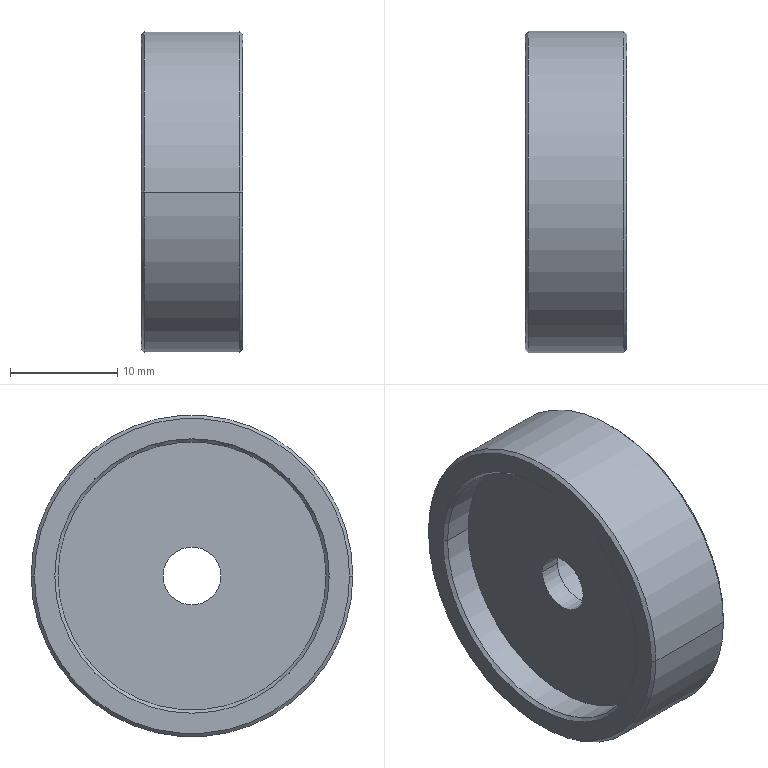Part | NX | 1 solid | 20 faces | box 9.5 x 30 x 30 mm | volume 4864 mm3 | cylinder 8 | cone 8 | plane 4 | commonest cylinder face diameters 5.4 x2 9.5 x2 25 x2 30 x2
STEP:
#1=CARTESIAN_POINT('',(215.3,157.591,-308.31));
#2=VERTEX_POINT('',#1);
#3=CARTESIAN_POINT('',(215.3,127.591,-308.31));
#4=VERTEX_POINT('',#3);
#5=CARTESIAN_POINT('',(215.3,142.591,-308.31));
#6=DIRECTION('',(-1.,0.,0.));
#7=DIRECTION('',(0.,-1.,0.));
#8=AXIS2_PLACEMENT_3D('',#5,#6,#7);
#9=CIRCLE('',#8,15.);
#10=EDGE_CURVE('',#2,#4,#9,.T.);
#11=ORIENTED_EDGE('',*,*,#10,.T.);
#12=CARTESIAN_POINT('',(206.4,127.591,-308.31));
#13=VERTEX_POINT('',#12);
#14=CARTESIAN_POINT('',(208.1,127.591,-308.31));
#15=DIRECTION('',(1.,0.,0.));
#16=VECTOR('',#15,1000.);
#17=LINE('',#14,#16);
#18=EDGE_CURVE('',#4,#13,#17,.F.);
#19=ORIENTED_EDGE('',*,*,#18,.T.);
#20=CARTESIAN_POINT('',(206.4,157.591,-308.31));
#21=VERTEX_POINT('',#20);
#22=CARTESIAN_POINT('',(206.4,142.591,-308.31));
#23=DIRECTION('',(1.,0.,0.));
#24=DIRECTION('',(0.,1.,0.));
#25=AXIS2_PLACEMENT_3D('',#22,#23,#24);
#26=CIRCLE('',#25,15.);
#27=EDGE_CURVE('',#13,#21,#26,.T.);
#28=ORIENTED_EDGE('',*,*,#27,.T.);
#29=CARTESIAN_POINT('',(208.1,157.591,-308.31));
#30=DIRECTION('',(1.,0.,0.));
#31=VECTOR('',#30,1000.);
#32=LINE('',#29,#31);
#33=EDGE_CURVE('',#2,#21,#32,.F.);
#34=ORIENTED_EDGE('',*,*,#33,.F.);
#35=EDGE_LOOP('',(#11,#19,#28,#34));
#36=FACE_BOUND('',#35,.T.);
#37=CARTESIAN_POINT('',(208.1,142.591,-308.31));
#38=DIRECTION('',(1.,0.,0.));
#39=DIRECTION('',(0.,1.,0.));
#40=AXIS2_PLACEMENT_3D('',#37,#38,#39);
#41=CYLINDRICAL_SURFACE('',#40,15.);
#42=ADVANCED_FACE('',(#36),#41,.T.);
#43=CARTESIAN_POINT('',(206.1,127.891,-308.31));
#44=VERTEX_POINT('',#43);
#45=CARTESIAN_POINT('',(206.1,157.291,-308.31));
#46=VERTEX_POINT('',#45);
#47=CARTESIAN_POINT('',(206.1,142.591,-308.31));
#48=DIRECTION('',(1.,0.,0.));
#49=DIRECTION('',(0.,1.,0.));
#50=AXIS2_PLACEMENT_3D('',#47,#48,#49);
#51=CIRCLE('',#50,14.7);
#52=EDGE_CURVE('',#44,#46,#51,.T.);
#53=ORIENTED_EDGE('',*,*,#52,.F.);
#54=CARTESIAN_POINT('',(206.1,142.591,-308.31));
#55=DIRECTION('',(1.,0.,0.));
#56=DIRECTION('',(0.,1.,0.));
#57=AXIS2_PLACEMENT_3D('',#54,#55,#56);
#58=CIRCLE('',#57,14.7);
#59=EDGE_CURVE('',#46,#44,#58,.T.);
#60=ORIENTED_EDGE('',*,*,#59,.F.);
#61=EDGE_LOOP('',(#53,#60));
#62=FACE_BOUND('',#61,.T.);
#63=CARTESIAN_POINT('',(206.1,129.791,-308.31));
#64=VERTEX_POINT('',#63);
#65=CARTESIAN_POINT('',(206.1,155.391,-308.31));
#66=VERTEX_POINT('',#65);
#67=CARTESIAN_POINT('',(206.1,142.591,-308.31));
#68=DIRECTION('',(-1.,0.,0.));
#69=DIRECTION('',(0.,-1.,0.));
#70=AXIS2_PLACEMENT_3D('',#67,#68,#69);
#71=CIRCLE('',#70,12.8);
#72=EDGE_CURVE('',#64,#66,#71,.T.);
#73=ORIENTED_EDGE('',*,*,#72,.F.);
#74=CARTESIAN_POINT('',(206.1,142.591,-308.31));
#75=DIRECTION('',(-1.,0.,0.));
#76=DIRECTION('',(0.,-1.,0.));
#77=AXIS2_PLACEMENT_3D('',#74,#75,#76);
#78=CIRCLE('',#77,12.8);
#79=EDGE_CURVE('',#66,#64,#78,.T.);
#80=ORIENTED_EDGE('',*,*,#79,.F.);
#81=EDGE_LOOP('',(#73,#80));
#82=FACE_BOUND('',#81,.T.);
#83=CARTESIAN_POINT('',(206.1,137.585,-304.813));
#84=DIRECTION('',(1.,0.,0.));
#85=DIRECTION('',(0.,1.,0.));
#86=AXIS2_PLACEMENT_3D('',#83,#84,#85);
#87=PLANE('',#86);
#88=ADVANCED_FACE('',(#62,#82),#87,.F.);
#89=ORIENTED_EDGE('',*,*,#72,.T.);
#90=CARTESIAN_POINT('',(206.4,155.091,-308.31));
#91=VERTEX_POINT('',#90);
#92=CARTESIAN_POINT('',(206.1,155.391,-308.31));
#93=DIRECTION('',(-0.7071,0.7071,0.));
#94=VECTOR('',#93,1000.);
#95=LINE('',#92,#94);
#96=EDGE_CURVE('',#91,#66,#95,.T.);
#97=ORIENTED_EDGE('',*,*,#96,.F.);
#98=CARTESIAN_POINT('',(206.4,130.091,-308.31));
#99=VERTEX_POINT('',#98);
#100=CARTESIAN_POINT('',(206.4,142.591,-308.31));
#101=DIRECTION('',(-1.,0.,0.));
#102=DIRECTION('',(0.,-1.,0.));
#103=AXIS2_PLACEMENT_3D('',#100,#101,#102);
#104=CIRCLE('',#103,12.5);
#105=EDGE_CURVE('',#99,#91,#104,.T.);
#106=ORIENTED_EDGE('',*,*,#105,.F.);
#107=CARTESIAN_POINT('',(206.1,129.791,-308.31));
#108=DIRECTION('',(-0.7071,-0.7071,0.));
#109=VECTOR('',#108,1000.);
#110=LINE('',#107,#109);
#111=EDGE_CURVE('',#99,#64,#110,.T.);
#112=ORIENTED_EDGE('',*,*,#111,.T.);
#113=EDGE_LOOP('',(#89,#97,#106,#112));
#114=FACE_BOUND('',#113,.T.);
#115=CARTESIAN_POINT('',(206.1,142.591,-308.31));
#116=DIRECTION('',(-1.,0.,0.));
#117=DIRECTION('',(0.,1.,0.));
#118=AXIS2_PLACEMENT_3D('',#115,#116,#117);
#119=CONICAL_SURFACE('',#118,12.8,0.7854);
#120=ADVANCED_FACE('',(#114),#119,.F.);
#121=CARTESIAN_POINT('',(206.4,142.591,-308.31));
#122=DIRECTION('',(1.,0.,0.));
#123=DIRECTION('',(0.,1.,0.));
#124=AXIS2_PLACEMENT_3D('',#121,#122,#123);
#125=CIRCLE('',#124,15.);
#126=EDGE_CURVE('',#21,#13,#125,.T.);
#127=ORIENTED_EDGE('',*,*,#126,.F.);
#128=CARTESIAN_POINT('',(206.1,157.291,-308.31));
#129=DIRECTION('',(0.7071,0.7071,0.));
#130=VECTOR('',#129,1000.);
#131=LINE('',#128,#130);
#132=EDGE_CURVE('',#46,#21,#131,.T.);
#133=ORIENTED_EDGE('',*,*,#132,.F.);
#134=ORIENTED_EDGE('',*,*,#59,.T.);
#135=CARTESIAN_POINT('',(206.1,127.891,-308.31));
#136=DIRECTION('',(0.7071,-0.7071,0.));
#137=VECTOR('',#136,1000.);
#138=LINE('',#135,#137);
#139=EDGE_CURVE('',#44,#13,#138,.T.);
#140=ORIENTED_EDGE('',*,*,#139,.T.);
#141=EDGE_LOOP('',(#127,#133,#134,#140));
#142=FACE_BOUND('',#141,.T.);
#143=CARTESIAN_POINT('',(206.1,142.591,-308.31));
#144=DIRECTION('',(1.,0.,0.));
#145=DIRECTION('',(0.,-1.,0.));
#146=AXIS2_PLACEMENT_3D('',#143,#144,#145);
#147=CONICAL_SURFACE('',#146,14.7,0.7854);
#148=ADVANCED_FACE('',(#142),#147,.T.);
#149=CARTESIAN_POINT('',(215.6,147.641,-308.31));
#150=VERTEX_POINT('',#149);
#151=CARTESIAN_POINT('',(215.6,137.541,-308.31));
#152=VERTEX_POINT('',#151);
#153=CARTESIAN_POINT('',(215.6,142.591,-308.31));
#154=DIRECTION('',(1.,0.,0.));
#155=DIRECTION('',(0.,1.,0.));
#156=AXIS2_PLACEMENT_3D('',#153,#154,#155);
#157=CIRCLE('',#156,5.05);
#158=EDGE_CURVE('',#150,#152,#157,.T.);
#159=ORIENTED_EDGE('',*,*,#158,.T.);
#160=CARTESIAN_POINT('',(215.3,137.841,-308.31));
#161=VERTEX_POINT('',#160);
#162=CARTESIAN_POINT('',(215.6,137.541,-308.31));
#163=DIRECTION('',(0.7071,-0.7071,0.));
#164=VECTOR('',#163,1000.);
#165=LINE('',#162,#164);
#166=EDGE_CURVE('',#152,#161,#165,.F.);
#167=ORIENTED_EDGE('',*,*,#166,.T.);
#168=CARTESIAN_POINT('',(215.3,147.341,-308.31));
#169=VERTEX_POINT('',#168);
#170=CARTESIAN_POINT('',(215.3,142.591,-308.31));
#171=DIRECTION('',(1.,0.,0.));
#172=DIRECTION('',(0.,1.,0.));
#173=AXIS2_PLACEMENT_3D('',#170,#171,#172);
#174=CIRCLE('',#173,4.75);
#175=EDGE_CURVE('',#169,#161,#174,.T.);
#176=ORIENTED_EDGE('',*,*,#175,.F.);
#177=CARTESIAN_POINT('',(215.6,147.641,-308.31));
#178=DIRECTION('',(0.7071,0.7071,0.));
#179=VECTOR('',#178,1000.);
#180=LINE('',#177,#179);
#181=EDGE_CURVE('',#150,#169,#180,.F.);
#182=ORIENTED_EDGE('',*,*,#181,.F.);
#183=EDGE_LOOP('',(#159,#167,#176,#182));
#184=FACE_BOUND('',#183,.T.);
#185=CARTESIAN_POINT('',(215.6,142.591,-308.31));
#186=DIRECTION('',(1.,0.,0.));
#187=DIRECTION('',(0.,-1.,0.));
#188=AXIS2_PLACEMENT_3D('',#185,#186,#187);
#189=CONICAL_SURFACE('',#188,5.05,0.7854);
#190=ADVANCED_FACE('',(#184),#189,.F.);
#191=ORIENTED_EDGE('',*,*,#10,.F.);
#192=CARTESIAN_POINT('',(215.6,157.291,-308.31));
#193=VERTEX_POINT('',#192);
#194=CARTESIAN_POINT('',(215.6,157.291,-308.31));
#195=DIRECTION('',(-0.7071,0.7071,0.));
#196=VECTOR('',#195,1000.);
#197=LINE('',#194,#196);
#198=EDGE_CURVE('',#193,#2,#197,.T.);
#199=ORIENTED_EDGE('',*,*,#198,.F.);
#200=CARTESIAN_POINT('',(215.6,127.891,-308.31));
#201=VERTEX_POINT('',#200);
#202=CARTESIAN_POINT('',(215.6,142.591,-308.31));
#203=DIRECTION('',(-1.,0.,0.));
#204=DIRECTION('',(0.,-1.,0.));
#205=AXIS2_PLACEMENT_3D('',#202,#203,#204);
#206=CIRCLE('',#205,14.7);
#207=EDGE_CURVE('',#193,#201,#206,.T.);
#208=ORIENTED_EDGE('',*,*,#207,.T.);
#209=CARTESIAN_POINT('',(215.6,127.891,-308.31));
#210=DIRECTION('',(-0.7071,-0.7071,0.));
#211=VECTOR('',#210,1000.);
#212=LINE('',#209,#211);
#213=EDGE_CURVE('',#201,#4,#212,.T.);
#214=ORIENTED_EDGE('',*,*,#213,.T.);
#215=EDGE_LOOP('',(#191,#199,#208,#214));
#216=FACE_BOUND('',#215,.T.);
#217=CARTESIAN_POINT('',(215.6,142.591,-308.31));
#218=DIRECTION('',(-1.,0.,0.));
#219=DIRECTION('',(0.,1.,0.));
#220=AXIS2_PLACEMENT_3D('',#217,#218,#219);
#221=CONICAL_SURFACE('',#220,14.7,0.7854);
#222=ADVANCED_FACE('',(#216),#221,.T.);
#223=CARTESIAN_POINT('',(211.1,147.341,-308.31));
#224=VERTEX_POINT('',#223);
#225=CARTESIAN_POINT('',(211.1,137.841,-308.31));
#226=VERTEX_POINT('',#225);
#227=CARTESIAN_POINT('',(211.1,142.591,-308.31));
#228=DIRECTION('',(1.,0.,0.));
#229=DIRECTION('',(0.,1.,0.));
#230=AXIS2_PLACEMENT_3D('',#227,#228,#229);
#231=CIRCLE('',#230,4.75);
#232=EDGE_CURVE('',#224,#226,#231,.T.);
#233=ORIENTED_EDGE('',*,*,#232,.T.);
#234=CARTESIAN_POINT('',(211.1,142.591,-308.31));
#235=DIRECTION('',(1.,0.,0.));
#236=DIRECTION('',(0.,1.,0.));
#237=AXIS2_PLACEMENT_3D('',#234,#235,#236);
#238=CIRCLE('',#237,4.75);
#239=EDGE_CURVE('',#226,#224,#238,.T.);
#240=ORIENTED_EDGE('',*,*,#239,.T.);
#241=EDGE_LOOP('',(#233,#240));
#242=FACE_BOUND('',#241,.T.);
#243=CARTESIAN_POINT('',(211.1,139.891,-308.31));
#244=VERTEX_POINT('',#243);
#245=CARTESIAN_POINT('',(211.1,145.291,-308.31));
#246=VERTEX_POINT('',#245);
#247=CARTESIAN_POINT('',(211.1,142.591,-308.31));
#248=DIRECTION('',(1.,0.,0.));
#249=DIRECTION('',(0.,1.,0.));
#250=AXIS2_PLACEMENT_3D('',#247,#248,#249);
#251=CIRCLE('',#250,2.7);
#252=EDGE_CURVE('',#244,#246,#251,.T.);
#253=ORIENTED_EDGE('',*,*,#252,.F.);
#254=CARTESIAN_POINT('',(211.1,142.591,-308.31));
#255=DIRECTION('',(1.,0.,0.));
#256=DIRECTION('',(0.,1.,0.));
#257=AXIS2_PLACEMENT_3D('',#254,#255,#256);
#258=CIRCLE('',#257,2.7);
#259=EDGE_CURVE('',#246,#244,#258,.T.);
#260=ORIENTED_EDGE('',*,*,#259,.F.);
#261=EDGE_LOOP('',(#253,#260));
#262=FACE_BOUND('',#261,.T.);
#263=CARTESIAN_POINT('',(211.1,140.554,-303.435));
#264=DIRECTION('',(1.,0.,0.));
#265=DIRECTION('',(0.,1.,0.));
#266=AXIS2_PLACEMENT_3D('',#263,#264,#265);
#267=PLANE('',#266);
#268=ADVANCED_FACE('',(#242,#262),#267,.T.);
#269=CARTESIAN_POINT('',(209.1,155.091,-308.31));
#270=VERTEX_POINT('',#269);
#271=CARTESIAN_POINT('',(209.1,130.091,-308.31));
#272=VERTEX_POINT('',#271);
#273=CARTESIAN_POINT('',(209.1,142.591,-308.31));
#274=DIRECTION('',(1.,0.,0.));
#275=DIRECTION('',(0.,1.,0.));
#276=AXIS2_PLACEMENT_3D('',#273,#274,#275);
#277=CIRCLE('',#276,12.5);
#278=EDGE_CURVE('',#270,#272,#277,.T.);
#279=ORIENTED_EDGE('',*,*,#278,.T.);
#280=CARTESIAN_POINT('',(208.1,130.091,-308.31));
#281=DIRECTION('',(1.,0.,0.));
#282=VECTOR('',#281,1000.);
#283=LINE('',#280,#282);
#284=EDGE_CURVE('',#99,#272,#283,.T.);
#285=ORIENTED_EDGE('',*,*,#284,.F.);
#286=ORIENTED_EDGE('',*,*,#105,.T.);
#287=CARTESIAN_POINT('',(208.1,155.091,-308.31));
#288=DIRECTION('',(1.,0.,0.));
#289=VECTOR('',#288,1000.);
#290=LINE('',#287,#289);
#291=EDGE_CURVE('',#91,#270,#290,.T.);
#292=ORIENTED_EDGE('',*,*,#291,.T.);
#293=EDGE_LOOP('',(#279,#285,#286,#292));
#294=FACE_BOUND('',#293,.T.);
#295=CARTESIAN_POINT('',(208.1,142.591,-308.31));
#296=DIRECTION('',(1.,0.,0.));
#297=DIRECTION('',(0.,1.,0.));
#298=AXIS2_PLACEMENT_3D('',#295,#296,#297);
#299=CYLINDRICAL_SURFACE('',#298,12.5);
#300=ADVANCED_FACE('',(#294),#299,.F.);
#301=CARTESIAN_POINT('',(215.6,142.591,-308.31));
#302=DIRECTION('',(-1.,0.,0.));
#303=DIRECTION('',(0.,-1.,0.));
#304=AXIS2_PLACEMENT_3D('',#301,#302,#303);
#305=CIRCLE('',#304,14.7);
#306=EDGE_CURVE('',#201,#193,#305,.T.);
#307=ORIENTED_EDGE('',*,*,#306,.F.);
#308=ORIENTED_EDGE('',*,*,#207,.F.);
#309=EDGE_LOOP('',(#307,#308));
#310=FACE_BOUND('',#309,.T.);
#311=ORIENTED_EDGE('',*,*,#158,.F.);
#312=CARTESIAN_POINT('',(215.6,142.591,-308.31));
#313=DIRECTION('',(1.,0.,0.));
#314=DIRECTION('',(0.,1.,0.));
#315=AXIS2_PLACEMENT_3D('',#312,#313,#314);
#316=CIRCLE('',#315,5.05);
#317=EDGE_CURVE('',#152,#150,#316,.T.);
#318=ORIENTED_EDGE('',*,*,#317,.F.);
#319=EDGE_LOOP('',(#311,#318));
#320=FACE_BOUND('',#319,.T.);
#321=CARTESIAN_POINT('',(215.6,137.585,-304.813));
#322=DIRECTION('',(1.,0.,0.));
#323=DIRECTION('',(0.,1.,0.));
#324=AXIS2_PLACEMENT_3D('',#321,#322,#323);
#325=PLANE('',#324);
#326=ADVANCED_FACE('',(#310,#320),#325,.T.);
#327=ORIENTED_EDGE('',*,*,#278,.F.);
#328=CARTESIAN_POINT('',(209.1,142.591,-308.31));
#329=DIRECTION('',(1.,0.,0.));
#330=DIRECTION('',(0.,1.,0.));
#331=AXIS2_PLACEMENT_3D('',#328,#329,#330);
#332=CIRCLE('',#331,12.5);
#333=EDGE_CURVE('',#272,#270,#332,.T.);
#334=ORIENTED_EDGE('',*,*,#333,.F.);
#335=EDGE_LOOP('',(#327,#334));
#336=FACE_BOUND('',#335,.T.);
#337=CARTESIAN_POINT('',(209.1,139.891,-308.31));
#338=VERTEX_POINT('',#337);
#339=CARTESIAN_POINT('',(209.1,145.291,-308.31));
#340=VERTEX_POINT('',#339);
#341=CARTESIAN_POINT('',(209.1,142.591,-308.31));
#342=DIRECTION('',(1.,0.,0.));
#343=DIRECTION('',(0.,1.,0.));
#344=AXIS2_PLACEMENT_3D('',#341,#342,#343);
#345=CIRCLE('',#344,2.7);
#346=EDGE_CURVE('',#338,#340,#345,.T.);
#347=ORIENTED_EDGE('',*,*,#346,.T.);
#348=CARTESIAN_POINT('',(209.1,142.591,-308.31));
#349=DIRECTION('',(1.,0.,0.));
#350=DIRECTION('',(0.,1.,0.));
#351=AXIS2_PLACEMENT_3D('',#348,#349,#350);
#352=CIRCLE('',#351,2.7);
#353=EDGE_CURVE('',#340,#338,#352,.T.);
#354=ORIENTED_EDGE('',*,*,#353,.T.);
#355=EDGE_LOOP('',(#347,#354));
#356=FACE_BOUND('',#355,.T.);
#357=CARTESIAN_POINT('',(209.1,137.585,-304.813));
#358=DIRECTION('',(1.,0.,0.));
#359=DIRECTION('',(0.,1.,0.));
#360=AXIS2_PLACEMENT_3D('',#357,#358,#359);
#361=PLANE('',#360);
#362=ADVANCED_FACE('',(#336,#356),#361,.F.);
#363=ORIENTED_EDGE('',*,*,#346,.F.);
#364=CARTESIAN_POINT('',(205.2,139.891,-308.31));
#365=DIRECTION('',(1.,0.,0.));
#366=VECTOR('',#365,1000.);
#367=LINE('',#364,#366);
#368=EDGE_CURVE('',#338,#244,#367,.T.);
#369=ORIENTED_EDGE('',*,*,#368,.T.);
#370=ORIENTED_EDGE('',*,*,#252,.T.);
#371=CARTESIAN_POINT('',(205.2,145.291,-308.31));
#372=DIRECTION('',(1.,0.,0.));
#373=VECTOR('',#372,1000.);
#374=LINE('',#371,#373);
#375=EDGE_CURVE('',#340,#246,#374,.T.);
#376=ORIENTED_EDGE('',*,*,#375,.F.);
#377=EDGE_LOOP('',(#363,#369,#370,#376));
#378=FACE_BOUND('',#377,.T.);
#379=CARTESIAN_POINT('',(205.2,142.591,-308.31));
#380=DIRECTION('',(1.,0.,0.));
#381=DIRECTION('',(0.,1.,0.));
#382=AXIS2_PLACEMENT_3D('',#379,#380,#381);
#383=CYLINDRICAL_SURFACE('',#382,2.7);
#384=ADVANCED_FACE('',(#378),#383,.F.);
#385=CARTESIAN_POINT('',(215.3,142.591,-308.31));
#386=DIRECTION('',(1.,0.,0.));
#387=DIRECTION('',(0.,1.,0.));
#388=AXIS2_PLACEMENT_3D('',#385,#386,#387);
#389=CIRCLE('',#388,4.75);
#390=EDGE_CURVE('',#161,#169,#389,.T.);
#391=ORIENTED_EDGE('',*,*,#390,.T.);
#392=CARTESIAN_POINT('',(215.1,147.341,-308.31));
#393=DIRECTION('',(1.,0.,0.));
#394=VECTOR('',#393,1000.);
#395=LINE('',#392,#394);
#396=EDGE_CURVE('',#224,#169,#395,.T.);
#397=ORIENTED_EDGE('',*,*,#396,.F.);
#398=ORIENTED_EDGE('',*,*,#239,.F.);
#399=CARTESIAN_POINT('',(215.1,137.841,-308.31));
#400=DIRECTION('',(1.,0.,0.));
#401=VECTOR('',#400,1000.);
#402=LINE('',#399,#401);
#403=EDGE_CURVE('',#226,#161,#402,.T.);
#404=ORIENTED_EDGE('',*,*,#403,.T.);
#405=EDGE_LOOP('',(#391,#397,#398,#404));
#406=FACE_BOUND('',#405,.T.);
#407=CARTESIAN_POINT('',(215.1,142.591,-308.31));
#408=DIRECTION('',(1.,0.,0.));
#409=DIRECTION('',(0.,1.,0.));
#410=AXIS2_PLACEMENT_3D('',#407,#408,#409);
#411=CYLINDRICAL_SURFACE('',#410,4.75);
#412=ADVANCED_FACE('',(#406),#411,.F.);
#413=ORIENTED_EDGE('',*,*,#232,.F.);
#414=ORIENTED_EDGE('',*,*,#396,.T.);
#415=ORIENTED_EDGE('',*,*,#175,.T.);
#416=ORIENTED_EDGE('',*,*,#403,.F.);
#417=EDGE_LOOP('',(#413,#414,#415,#416));
#418=FACE_BOUND('',#417,.T.);
#419=CARTESIAN_POINT('',(215.1,142.591,-308.31));
#420=DIRECTION('',(1.,0.,0.));
#421=DIRECTION('',(0.,1.,0.));
#422=AXIS2_PLACEMENT_3D('',#419,#420,#421);
#423=CYLINDRICAL_SURFACE('',#422,4.75);
#424=ADVANCED_FACE('',(#418),#423,.F.);
#425=ORIENTED_EDGE('',*,*,#52,.T.);
#426=ORIENTED_EDGE('',*,*,#132,.T.);
#427=ORIENTED_EDGE('',*,*,#27,.F.);
#428=ORIENTED_EDGE('',*,*,#139,.F.);
#429=EDGE_LOOP('',(#425,#426,#427,#428));
#430=FACE_BOUND('',#429,.T.);
#431=CARTESIAN_POINT('',(206.1,142.591,-308.31));
#432=DIRECTION('',(1.,0.,0.));
#433=DIRECTION('',(0.,-1.,0.));
#434=AXIS2_PLACEMENT_3D('',#431,#432,#433);
#435=CONICAL_SURFACE('',#434,14.7,0.7854);
#436=ADVANCED_FACE('',(#430),#435,.T.);
#437=ORIENTED_EDGE('',*,*,#390,.F.);
#438=ORIENTED_EDGE('',*,*,#166,.F.);
#439=ORIENTED_EDGE('',*,*,#317,.T.);
#440=ORIENTED_EDGE('',*,*,#181,.T.);
#441=EDGE_LOOP('',(#437,#438,#439,#440));
#442=FACE_BOUND('',#441,.T.);
#443=CARTESIAN_POINT('',(215.6,142.591,-308.31));
#444=DIRECTION('',(1.,0.,0.));
#445=DIRECTION('',(0.,-1.,0.));
#446=AXIS2_PLACEMENT_3D('',#443,#444,#445);
#447=CONICAL_SURFACE('',#446,5.05,0.7854);
#448=ADVANCED_FACE('',(#442),#447,.F.);
#449=ORIENTED_EDGE('',*,*,#96,.T.);
#450=ORIENTED_EDGE('',*,*,#79,.T.);
#451=ORIENTED_EDGE('',*,*,#111,.F.);
#452=CARTESIAN_POINT('',(206.4,142.591,-308.31));
#453=DIRECTION('',(-1.,0.,0.));
#454=DIRECTION('',(0.,-1.,0.));
#455=AXIS2_PLACEMENT_3D('',#452,#453,#454);
#456=CIRCLE('',#455,12.5);
#457=EDGE_CURVE('',#91,#99,#456,.T.);
#458=ORIENTED_EDGE('',*,*,#457,.F.);
#459=EDGE_LOOP('',(#449,#450,#451,#458));
#460=FACE_BOUND('',#459,.T.);
#461=CARTESIAN_POINT('',(206.1,142.591,-308.31));
#462=DIRECTION('',(-1.,0.,0.));
#463=DIRECTION('',(0.,1.,0.));
#464=AXIS2_PLACEMENT_3D('',#461,#462,#463);
#465=CONICAL_SURFACE('',#464,12.8,0.7854);
#466=ADVANCED_FACE('',(#460),#465,.F.);
#467=ORIENTED_EDGE('',*,*,#291,.F.);
#468=ORIENTED_EDGE('',*,*,#457,.T.);
#469=ORIENTED_EDGE('',*,*,#284,.T.);
#470=ORIENTED_EDGE('',*,*,#333,.T.);
#471=EDGE_LOOP('',(#467,#468,#469,#470));
#472=FACE_BOUND('',#471,.T.);
#473=CARTESIAN_POINT('',(208.1,142.591,-308.31));
#474=DIRECTION('',(1.,0.,0.));
#475=DIRECTION('',(0.,1.,0.));
#476=AXIS2_PLACEMENT_3D('',#473,#474,#475);
#477=CYLINDRICAL_SURFACE('',#476,12.5);
#478=ADVANCED_FACE('',(#472),#477,.F.);
#479=ORIENTED_EDGE('',*,*,#306,.T.);
#480=ORIENTED_EDGE('',*,*,#198,.T.);
#481=CARTESIAN_POINT('',(215.3,142.591,-308.31));
#482=DIRECTION('',(-1.,0.,0.));
#483=DIRECTION('',(0.,-1.,0.));
#484=AXIS2_PLACEMENT_3D('',#481,#482,#483);
#485=CIRCLE('',#484,15.);
#486=EDGE_CURVE('',#4,#2,#485,.T.);
#487=ORIENTED_EDGE('',*,*,#486,.F.);
#488=ORIENTED_EDGE('',*,*,#213,.F.);
#489=EDGE_LOOP('',(#479,#480,#487,#488));
#490=FACE_BOUND('',#489,.T.);
#491=CARTESIAN_POINT('',(215.6,142.591,-308.31));
#492=DIRECTION('',(-1.,0.,0.));
#493=DIRECTION('',(0.,1.,0.));
#494=AXIS2_PLACEMENT_3D('',#491,#492,#493);
#495=CONICAL_SURFACE('',#494,14.7,0.7854);
#496=ADVANCED_FACE('',(#490),#495,.T.);
#497=ORIENTED_EDGE('',*,*,#126,.T.);
#498=ORIENTED_EDGE('',*,*,#18,.F.);
#499=ORIENTED_EDGE('',*,*,#486,.T.);
#500=ORIENTED_EDGE('',*,*,#33,.T.);
#501=EDGE_LOOP('',(#497,#498,#499,#500));
#502=FACE_BOUND('',#501,.T.);
#503=CARTESIAN_POINT('',(208.1,142.591,-308.31));
#504=DIRECTION('',(1.,0.,0.));
#505=DIRECTION('',(0.,1.,0.));
#506=AXIS2_PLACEMENT_3D('',#503,#504,#505);
#507=CYLINDRICAL_SURFACE('',#506,15.);
#508=ADVANCED_FACE('',(#502),#507,.T.);
#509=ORIENTED_EDGE('',*,*,#375,.T.);
#510=ORIENTED_EDGE('',*,*,#259,.T.);
#511=ORIENTED_EDGE('',*,*,#368,.F.);
#512=ORIENTED_EDGE('',*,*,#353,.F.);
#513=EDGE_LOOP('',(#509,#510,#511,#512));
#514=FACE_BOUND('',#513,.T.);
#515=CARTESIAN_POINT('',(205.2,142.591,-308.31));
#516=DIRECTION('',(1.,0.,0.));
#517=DIRECTION('',(0.,1.,0.));
#518=AXIS2_PLACEMENT_3D('',#515,#516,#517);
#519=CYLINDRICAL_SURFACE('',#518,2.7);
#520=ADVANCED_FACE('',(#514),#519,.F.);
#521=CLOSED_SHELL('',(#42,#88,#120,#148,#190,#222,#268,#300,#326,#362,#384,#412,#424,#436,#448,#466,#478,#496,#508,#520));
#522=MANIFOLD_SOLID_BREP('',#521);
#523=(LENGTH_UNIT()NAMED_UNIT(*)SI_UNIT(.MILLI.,.METRE.));
#524=UNCERTAINTY_MEASURE_WITH_UNIT(LENGTH_MEASURE(0.00001),#523,'','');
#525=(NAMED_UNIT(*)PLANE_ANGLE_UNIT()SI_UNIT($,.RADIAN.));
#526=(NAMED_UNIT(*)SI_UNIT($,.STERADIAN.)SOLID_ANGLE_UNIT());
#527=(GEOMETRIC_REPRESENTATION_CONTEXT(3)GLOBAL_UNCERTAINTY_ASSIGNED_CONTEXT((#524))GLOBAL_UNIT_ASSIGNED_CONTEXT((#523,#525,#526))REPRESENTATION_CONTEXT('',''));
#528=ADVANCED_BREP_SHAPE_REPRESENTATION('',(#522),#527);